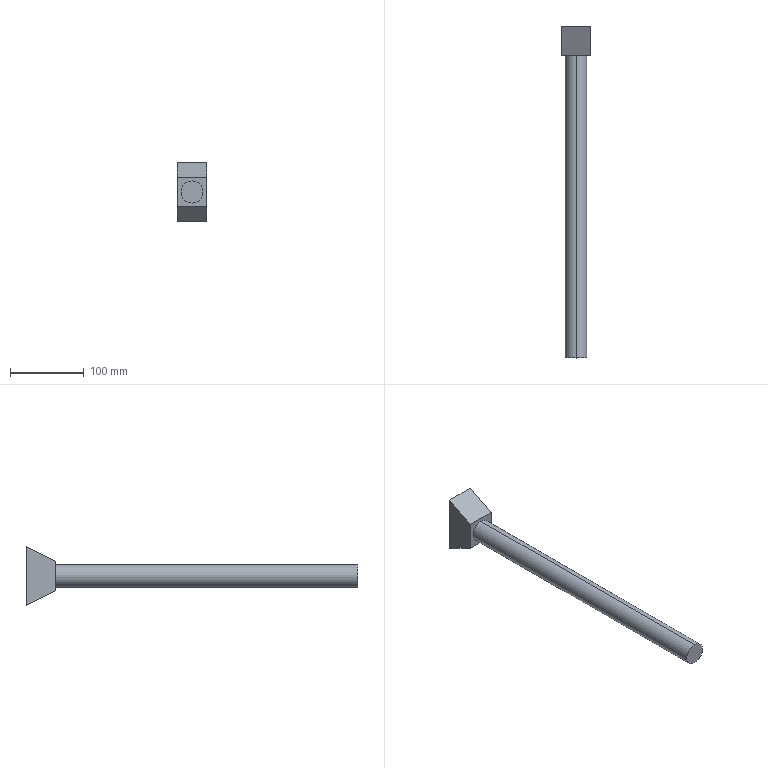Part | SolidWorks | features ICE 2, Extrusion 1 | 1 solid | 9 faces | box 40 x 450 x 80 mm | volume 385812 mm3 | plane 7 | cylinder 2 | commonest cylinder face diameters 30 x2
STEP:
#1=CARTESIAN_POINT('',(0.,-430.,-15.));
#2=VERTEX_POINT('',#1);
#3=CARTESIAN_POINT('',(0.,-430.,15.));
#4=VERTEX_POINT('',#3);
#5=CARTESIAN_POINT('',(0.,-430.,0.));
#6=DIRECTION('',(0.,-1.,0.));
#7=DIRECTION('',(0.,0.,-1.));
#8=AXIS2_PLACEMENT_3D('',#5,#6,#7);
#9=CIRCLE('',#8,15.);
#10=EDGE_CURVE('',#2,#4,#9,.T.);
#11=ORIENTED_EDGE('',*,*,#10,.F.);
#12=CARTESIAN_POINT('',(0.,-20.,-15.));
#13=VERTEX_POINT('',#12);
#14=CARTESIAN_POINT('',(0.,-430.,-15.));
#15=DIRECTION('',(0.,1.,0.));
#16=VECTOR('',#15,1000.);
#17=LINE('',#14,#16);
#18=EDGE_CURVE('',#2,#13,#17,.T.);
#19=ORIENTED_EDGE('',*,*,#18,.T.);
#20=CARTESIAN_POINT('',(0.,-20.,15.));
#21=VERTEX_POINT('',#20);
#22=CARTESIAN_POINT('',(0.,-20.,0.));
#23=DIRECTION('',(0.,-1.,0.));
#24=DIRECTION('',(0.,0.,1.));
#25=AXIS2_PLACEMENT_3D('',#22,#23,#24);
#26=CIRCLE('',#25,15.);
#27=EDGE_CURVE('',#13,#21,#26,.T.);
#28=ORIENTED_EDGE('',*,*,#27,.T.);
#29=CARTESIAN_POINT('',(0.,-430.,15.));
#30=DIRECTION('',(0.,1.,0.));
#31=VECTOR('',#30,1000.);
#32=LINE('',#29,#31);
#33=EDGE_CURVE('',#4,#21,#32,.T.);
#34=ORIENTED_EDGE('',*,*,#33,.F.);
#35=EDGE_LOOP('',(#11,#19,#28,#34));
#36=FACE_OUTER_BOUND('',#35,.T.);
#37=CARTESIAN_POINT('',(0.,-430.,0.));
#38=DIRECTION('',(0.,1.,0.));
#39=DIRECTION('',(0.,0.,1.));
#40=AXIS2_PLACEMENT_3D('',#37,#38,#39);
#41=CYLINDRICAL_SURFACE('',#40,15.);
#42=ADVANCED_FACE('',(#36),#41,.T.);
#43=CARTESIAN_POINT('',(0.,-20.,0.));
#44=DIRECTION('',(0.,-1.,0.));
#45=DIRECTION('',(0.,0.,1.));
#46=AXIS2_PLACEMENT_3D('',#43,#44,#45);
#47=CIRCLE('',#46,15.);
#48=EDGE_CURVE('',#21,#13,#47,.T.);
#49=ORIENTED_EDGE('',*,*,#48,.F.);
#50=ORIENTED_EDGE('',*,*,#27,.F.);
#51=EDGE_LOOP('',(#49,#50));
#52=FACE_BOUND('',#51,.T.);
#53=CARTESIAN_POINT('',(-20.,-20.,20.));
#54=VERTEX_POINT('',#53);
#55=CARTESIAN_POINT('',(-20.,-20.,-20.));
#56=VERTEX_POINT('',#55);
#57=CARTESIAN_POINT('',(-20.,-20.,-40.));
#58=DIRECTION('',(0.,0.,-1.));
#59=VECTOR('',#58,1000.);
#60=LINE('',#57,#59);
#61=EDGE_CURVE('',#54,#56,#60,.T.);
#62=ORIENTED_EDGE('',*,*,#61,.T.);
#63=CARTESIAN_POINT('',(20.,-20.,-20.));
#64=VERTEX_POINT('',#63);
#65=CARTESIAN_POINT('',(-20.,-20.,-20.));
#66=DIRECTION('',(1.,0.,0.));
#67=VECTOR('',#66,1000.);
#68=LINE('',#65,#67);
#69=EDGE_CURVE('',#56,#64,#68,.T.);
#70=ORIENTED_EDGE('',*,*,#69,.T.);
#71=CARTESIAN_POINT('',(20.,-20.,20.));
#72=VERTEX_POINT('',#71);
#73=CARTESIAN_POINT('',(20.,-20.,-40.));
#74=DIRECTION('',(0.,0.,-1.));
#75=VECTOR('',#74,1000.);
#76=LINE('',#73,#75);
#77=EDGE_CURVE('',#72,#64,#76,.T.);
#78=ORIENTED_EDGE('',*,*,#77,.F.);
#79=CARTESIAN_POINT('',(-20.,-20.,20.));
#80=DIRECTION('',(1.,0.,0.));
#81=VECTOR('',#80,1000.);
#82=LINE('',#79,#81);
#83=EDGE_CURVE('',#54,#72,#82,.T.);
#84=ORIENTED_EDGE('',*,*,#83,.F.);
#85=EDGE_LOOP('',(#62,#70,#78,#84));
#86=FACE_OUTER_BOUND('',#85,.T.);
#87=CARTESIAN_POINT('',(20.,-20.,-40.));
#88=DIRECTION('',(0.,1.,0.));
#89=DIRECTION('',(0.,0.,1.));
#90=AXIS2_PLACEMENT_3D('',#87,#88,#89);
#91=PLANE('',#90);
#92=ADVANCED_FACE('',(#52,#86),#91,.F.);
#93=CARTESIAN_POINT('',(-20.,20.,-40.));
#94=VERTEX_POINT('',#93);
#95=CARTESIAN_POINT('',(-20.,20.,40.));
#96=VERTEX_POINT('',#95);
#97=CARTESIAN_POINT('',(-20.,20.,-40.));
#98=DIRECTION('',(0.,0.,1.));
#99=VECTOR('',#98,1000.);
#100=LINE('',#97,#99);
#101=EDGE_CURVE('',#94,#96,#100,.T.);
#102=ORIENTED_EDGE('',*,*,#101,.T.);
#103=CARTESIAN_POINT('',(20.,20.,40.));
#104=VERTEX_POINT('',#103);
#105=CARTESIAN_POINT('',(20.,20.,40.));
#106=DIRECTION('',(-1.,0.,0.));
#107=VECTOR('',#106,1000.);
#108=LINE('',#105,#107);
#109=EDGE_CURVE('',#104,#96,#108,.T.);
#110=ORIENTED_EDGE('',*,*,#109,.F.);
#111=CARTESIAN_POINT('',(20.,20.,-40.));
#112=VERTEX_POINT('',#111);
#113=CARTESIAN_POINT('',(20.,20.,-40.));
#114=DIRECTION('',(0.,0.,1.));
#115=VECTOR('',#114,1000.);
#116=LINE('',#113,#115);
#117=EDGE_CURVE('',#112,#104,#116,.T.);
#118=ORIENTED_EDGE('',*,*,#117,.F.);
#119=CARTESIAN_POINT('',(20.,20.,-40.));
#120=DIRECTION('',(-1.,0.,0.));
#121=VECTOR('',#120,1000.);
#122=LINE('',#119,#121);
#123=EDGE_CURVE('',#112,#94,#122,.T.);
#124=ORIENTED_EDGE('',*,*,#123,.T.);
#125=EDGE_LOOP('',(#102,#110,#118,#124));
#126=FACE_OUTER_BOUND('',#125,.T.);
#127=CARTESIAN_POINT('',(20.,20.,-40.));
#128=DIRECTION('',(0.,-1.,0.));
#129=DIRECTION('',(0.,0.,-1.));
#130=AXIS2_PLACEMENT_3D('',#127,#128,#129);
#131=PLANE('',#130);
#132=ADVANCED_FACE('',(#126),#131,.F.);
#133=CARTESIAN_POINT('',(20.,-20.,-20.));
#134=DIRECTION('',(0.,-0.8944,0.4472));
#135=VECTOR('',#134,1000.);
#136=LINE('',#133,#135);
#137=EDGE_CURVE('',#112,#64,#136,.T.);
#138=ORIENTED_EDGE('',*,*,#137,.F.);
#139=ORIENTED_EDGE('',*,*,#117,.T.);
#140=CARTESIAN_POINT('',(20.,20.,40.));
#141=DIRECTION('',(0.,0.8944,0.4472));
#142=VECTOR('',#141,1000.);
#143=LINE('',#140,#142);
#144=EDGE_CURVE('',#72,#104,#143,.T.);
#145=ORIENTED_EDGE('',*,*,#144,.F.);
#146=ORIENTED_EDGE('',*,*,#77,.T.);
#147=EDGE_LOOP('',(#138,#139,#145,#146));
#148=FACE_OUTER_BOUND('',#147,.T.);
#149=CARTESIAN_POINT('',(20.,0.,0.));
#150=DIRECTION('',(1.,0.,0.));
#151=DIRECTION('',(0.,0.,-1.));
#152=AXIS2_PLACEMENT_3D('',#149,#150,#151);
#153=PLANE('',#152);
#154=ADVANCED_FACE('',(#148),#153,.T.);
#155=ORIENTED_EDGE('',*,*,#101,.F.);
#156=CARTESIAN_POINT('',(-20.,-20.,-20.));
#157=DIRECTION('',(0.,-0.8944,0.4472));
#158=VECTOR('',#157,1000.);
#159=LINE('',#156,#158);
#160=EDGE_CURVE('',#94,#56,#159,.T.);
#161=ORIENTED_EDGE('',*,*,#160,.T.);
#162=ORIENTED_EDGE('',*,*,#61,.F.);
#163=CARTESIAN_POINT('',(-20.,20.,40.));
#164=DIRECTION('',(0.,0.8944,0.4472));
#165=VECTOR('',#164,1000.);
#166=LINE('',#163,#165);
#167=EDGE_CURVE('',#54,#96,#166,.T.);
#168=ORIENTED_EDGE('',*,*,#167,.T.);
#169=EDGE_LOOP('',(#155,#161,#162,#168));
#170=FACE_OUTER_BOUND('',#169,.T.);
#171=CARTESIAN_POINT('',(-20.,0.,0.));
#172=DIRECTION('',(1.,0.,0.));
#173=DIRECTION('',(0.,0.,-1.));
#174=AXIS2_PLACEMENT_3D('',#171,#172,#173);
#175=PLANE('',#174);
#176=ADVANCED_FACE('',(#170),#175,.F.);
#177=ORIENTED_EDGE('',*,*,#109,.T.);
#178=ORIENTED_EDGE('',*,*,#167,.F.);
#179=ORIENTED_EDGE('',*,*,#83,.T.);
#180=ORIENTED_EDGE('',*,*,#144,.T.);
#181=EDGE_LOOP('',(#177,#178,#179,#180));
#182=FACE_OUTER_BOUND('',#181,.T.);
#183=CARTESIAN_POINT('',(-20.,20.,40.));
#184=DIRECTION('',(0.,0.4472,-0.8944));
#185=DIRECTION('',(0.,0.8944,0.4472));
#186=AXIS2_PLACEMENT_3D('',#183,#184,#185);
#187=PLANE('',#186);
#188=ADVANCED_FACE('',(#182),#187,.F.);
#189=ORIENTED_EDGE('',*,*,#69,.F.);
#190=ORIENTED_EDGE('',*,*,#160,.F.);
#191=ORIENTED_EDGE('',*,*,#123,.F.);
#192=ORIENTED_EDGE('',*,*,#137,.T.);
#193=EDGE_LOOP('',(#189,#190,#191,#192));
#194=FACE_OUTER_BOUND('',#193,.T.);
#195=CARTESIAN_POINT('',(-20.,-20.,-20.));
#196=DIRECTION('',(0.,0.4472,0.8944));
#197=DIRECTION('',(0.,-0.8944,0.4472));
#198=AXIS2_PLACEMENT_3D('',#195,#196,#197);
#199=PLANE('',#198);
#200=ADVANCED_FACE('',(#194),#199,.F.);
#201=ORIENTED_EDGE('',*,*,#18,.F.);
#202=CARTESIAN_POINT('',(0.,-430.,0.));
#203=DIRECTION('',(0.,-1.,0.));
#204=DIRECTION('',(0.,0.,-1.));
#205=AXIS2_PLACEMENT_3D('',#202,#203,#204);
#206=CIRCLE('',#205,15.);
#207=EDGE_CURVE('',#4,#2,#206,.T.);
#208=ORIENTED_EDGE('',*,*,#207,.F.);
#209=ORIENTED_EDGE('',*,*,#33,.T.);
#210=ORIENTED_EDGE('',*,*,#48,.T.);
#211=EDGE_LOOP('',(#201,#208,#209,#210));
#212=FACE_OUTER_BOUND('',#211,.T.);
#213=CARTESIAN_POINT('',(0.,-430.,0.));
#214=DIRECTION('',(0.,1.,0.));
#215=DIRECTION('',(0.,0.,1.));
#216=AXIS2_PLACEMENT_3D('',#213,#214,#215);
#217=CYLINDRICAL_SURFACE('',#216,15.);
#218=ADVANCED_FACE('',(#212),#217,.T.);
#219=ORIENTED_EDGE('',*,*,#207,.T.);
#220=ORIENTED_EDGE('',*,*,#10,.T.);
#221=EDGE_LOOP('',(#219,#220));
#222=FACE_OUTER_BOUND('',#221,.T.);
#223=CARTESIAN_POINT('',(0.,-430.,0.));
#224=DIRECTION('',(0.,-1.,0.));
#225=DIRECTION('',(0.,0.,-1.));
#226=AXIS2_PLACEMENT_3D('',#223,#224,#225);
#227=PLANE('',#226);
#228=ADVANCED_FACE('',(#222),#227,.T.);
#229=CLOSED_SHELL('',(#42,#92,#132,#154,#176,#188,#200,#218,#228));
#230=MANIFOLD_SOLID_BREP('',#229);
#231=CARTESIAN_POINT('',(0.,0.,0.));
#232=DIRECTION('',(0.,0.,1.));
#233=DIRECTION('',(1.,0.,0.));
#234=AXIS2_PLACEMENT_3D('',#231,#232,#233);
#235=(LENGTH_UNIT()NAMED_UNIT(*)SI_UNIT(.MILLI.,.METRE.));
#236=UNCERTAINTY_MEASURE_WITH_UNIT(LENGTH_MEASURE(0.00001),#235,'','');
#237=(NAMED_UNIT(*)PLANE_ANGLE_UNIT()SI_UNIT($,.RADIAN.));
#238=(NAMED_UNIT(*)SI_UNIT($,.STERADIAN.)SOLID_ANGLE_UNIT());
#239=(GEOMETRIC_REPRESENTATION_CONTEXT(3)GLOBAL_UNCERTAINTY_ASSIGNED_CONTEXT((#236))GLOBAL_UNIT_ASSIGNED_CONTEXT((#235,#237,#238))REPRESENTATION_CONTEXT('',''));
#240=ADVANCED_BREP_SHAPE_REPRESENTATION('',(#230,#234),#239);